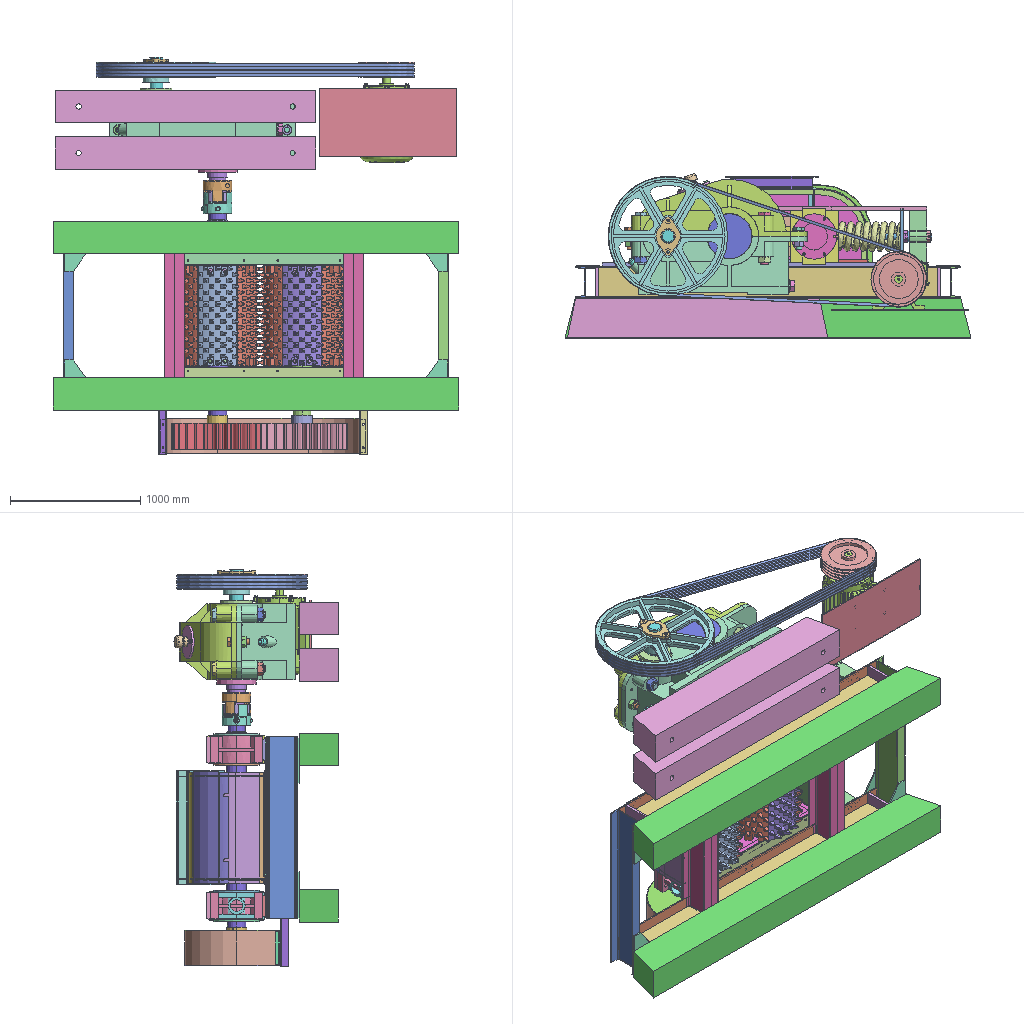Assembly | NX | 107 different items | 209 placed | box 3120 x 1261 x 3058 mm
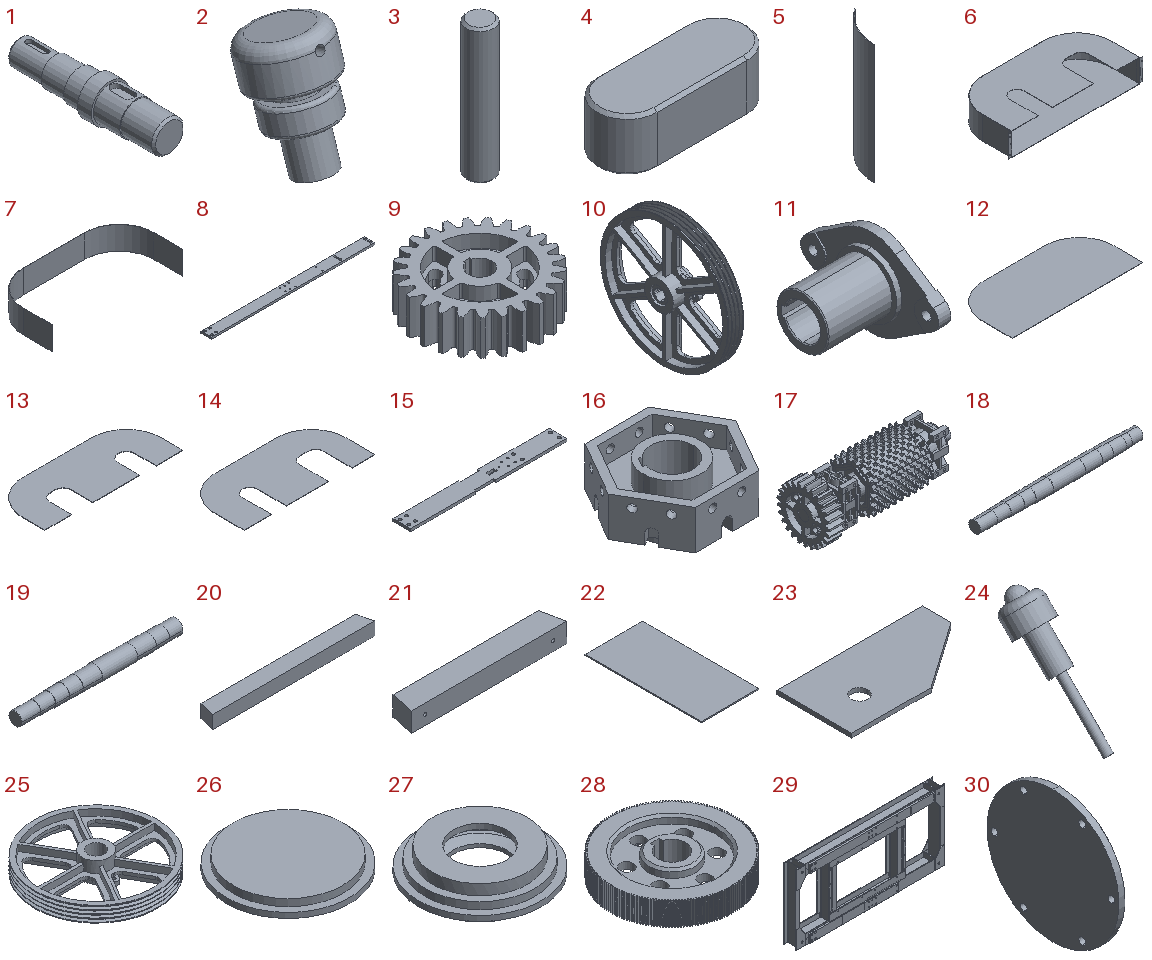Parts list (item | name | quantity | parent item | size | volume | features):
1 | - | x1 | in 84 | 202.5 x 798.75 x 202.5 mm | 16646925 mm3 | features BOSS 5, CHAMFER 2, DATUM_PLANE 2, RECT_SLOT 2, CYLINDER 1, DATUM_CSYS 1, Delete Body 1, LINKED_BODY 1, MOVE_FACE 1, SCALE 1
2 | - | x1 | in 84 | 93.696 x 105.756 x 150.047 mm | 549540 mm3 | features LINKED_BODY 2, DATUM_CSYS 1, Delete Body 1, Resize Face 1
3 | - | x1 | in 84 | 16.875 x 16.875 x 84.375 mm | 18772 mm3 | features LINKED_BODY 2, DATUM_CSYS 1, Delete Body 1
4 | - | x1 | in 84 | 112.5 x 45 x 39.375 mm | 180850 mm3 | features 28.SLDPRT 2, Delete Body 1, LINKED_BODY 1, SCALE 1
5 | - | x2 | in 75 | 160.623 x 300.85 x 860 mm | 907934 mm3 | features BREP 1
6 | - | x1 | - | 1570 x 734 x 271 mm | 7806699 mm3 | features BREP 4, DATUM_CSYS 1, SKETCH 1
7 | - | x1 | in 6 | 1498 x 729 x 265 mm | 2073983 mm3 | features BREP 1
8 | - | x1 | in 29 | 2499 x 158 x 30 mm | 11579104 mm3 | features BREP 1
9 | - | x2 | in 17, 65 | 701.605 x 700.371 x 200 mm | 42253808 mm3 | features BREP 1
10 | - | x1 | - | 178.109 x 915.408 x 915.408 mm | 21519028 mm3 | features BREP 2, SCALE 2, SPLIT BODY 1, UNITE 1
11 | - | x1 | in 10 | 171.496 x 296.82 x 187.986 mm | 1461921 mm3 | features BREP 1, SCALE 1
12 | - | x1 | in 6 | 1492 x 726 x 3 mm | 3047658 mm3 | features BREP 1, DATUM_CSYS 1, SKETCH 1
13 | - | x2 | in 75 | 1420 x 580 x 4 mm | 2620909 mm3 | features BREP 1
14 | - | x1 | in 6 | 1492 x 726 x 3 mm | 2518464 mm3 | features BREP 1
15 | - | x2 | - | 1759 x 200 x 30 mm | 9929100 mm3 | features BREP 1, DATUM_CSYS 1, SKETCH 1
16 | - | x4 | in 17, 65 | 484.974 x 420 x 200 mm | 14525982 mm3 | features BREP 1
17 | - | x1 | - | - | 267145378 mm3 | features BREP 14, MOVE_FACE 4, DATUM_CSYS 3, SKETCH 3
18 | - | x1 | in 17 | 1889 x 162.539 x 165 mm | 34030029 mm3 | features MOVE_FACE 3, BREP 1
19 | - | x1 | in 65 | 1692 x 162.539 x 165 mm | 31180686 mm3 | features BREP 1
20 | - | x2 | - | 3120 x 300 x 250 mm | 228112500 mm3 | features DATUM_CSYS 1, EXTRUDE 1, SKETCH 1
21 | - | x2 | - | 2000 x 300 x 250 mm | 144558518 mm3 | features BREP 1
22 | - | x1 | - | 525 x 1060 x 10 mm | 5565000 mm3 | features MOVE_FACE 3, BREP 1, DATUM_CSYS 1, DELETE FACE 1, SKETCH 1
23 | - | x8 | in 29 | 350 x 180 x 10 mm | 527834 mm3 | features BREP 1, DATUM_CSYS 1, SKETCH 1
24 | - | x1 | in 84 | 57.861 x 160.996 x 160.996 mm | 163265 mm3 | features DATUM_CSYS 2, Delete Body 2, LINKED_BODY 2, BLEND 1, DATUM_PLANE 1, SCALE 1, SKETCH 1, SWP104 1
25 | - | x1 | in 10 | 915.408 x 915.408 x 151.725 mm | 20057107 mm3 | features BREP 1, SCALE 1, SPLIT BODY 1, UNITE 1
26 | - | x1 | in 84 | 393.75 x 393.75 x 39.375 mm | 3155764 mm3 | features CYLINDER 3, DATUM_CSYS 1, Delete Body 1, LINKED_BODY 1, SCALE 1
27 | - | x1 | in 84 | 393.75 x 393.75 x 90 mm | 4276272 mm3 | features SIMPLE HOLE 4, CYLINDER 3, CHAMFER 2, DATUM_CSYS 1, Delete Body 1, LINKED_BODY 1, SCALE 1
28 | - | x1 | in 84 | 784.688 x 784.688 x 146.25 mm | 44829602 mm3 | features BREP 184, META 184, INSTANCE 55, EXTRUDE 6, SKETCH 4, CHAMFER 2, CYLINDER 2, DATUM_CSYS 2, Delete Body 2, EXTRACT_FACE 2, CIRCULAR_ISET 1, FSET 1, Instance Feature 1, LINKED_BODY 1, Mirror Feature 1, REPLACE_FACE 1, Resize Face 1, SCALE 1, SWP104 1, TRANSFORM_ISET 1
29 | - | x1 | - | 2963 x 280 x 1400 mm | 109819651 mm3 | features BREP 14, DATUM_CSYS 3, SKETCH 3, LINKED_FACE 1, REPLACE_FACE 1
30 | - | x1 | in 65 | 45 x 350 x 350 mm | 1642719 mm3 | features BREP 1
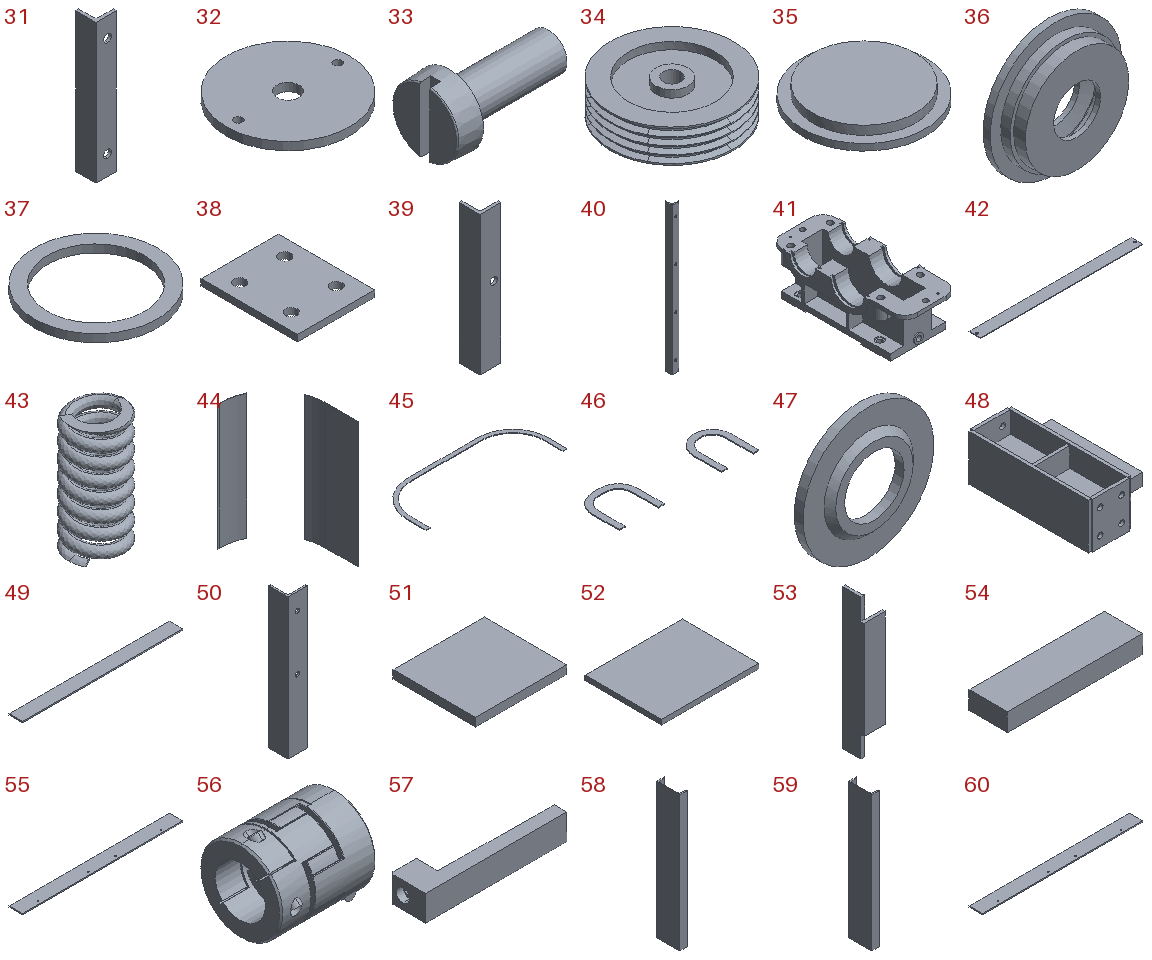31 | - | x2 | in 6 | 36 x 36 x 250 mm | 83297 mm3 | features BREP 1
32 | - | x1 | in 84 | - | 851530 mm3 | features Delete Body 2, LINKED_BODY 2, SIMPLE HOLE 2, SYMBOLIC_THREAD 2, CYLINDER 1, DATUM_CSYS 1, MIRROR_SET 1, SCALE 1, SUBTRACT 1
33 | - | x2 | in 84 | 56.25 x 30.938 x 30.938 mm | 17558 mm3 | features 7.SLDPRT 2, Delete Body 1, LINKED_BODY 1, MOVE_FACE 1, SCALE 1
34 | - | x1 | - | 426.001 x 426 x 114.878 mm | 11128143 mm3 | features DATUM_CSYS 1, LINKED_BODY 1
35 | - | x1 | in 84 | 315 x 315 x 39.375 mm | 2172802 mm3 | features CYLINDER 3, DATUM_CSYS 1, Delete Body 1, LINKED_BODY 1, SCALE 1, UNITE 1
36 | - | x1 | in 84 | 315 x 84.375 x 315 mm | 2887099 mm3 | features SIMPLE HOLE 4, CHAMFER 3, DATUM_CSYS 1, Delete Body 1, LINKED_BODY 1, SCALE 1, SKETCH 1, SWP104 1
37 | - | x2 | in 84 | 264.375 x 264.375 x 16.875 mm | 352256 mm3 | features CYLINDER 2, DATUM_CSYS 1, Delete Body 1, LINKED_BODY 1, SCALE 1
38 | - | x4 | in 48 | 120 x 150 x 10 mm | 169821 mm3 | features BREP 1
39 | - | x2 | in 75 | 40 x 40 x 270 mm | 101929 mm3 | features BREP 1
40 | - | x2 | in 75 | 40 x 40 x 850 mm | 320232 mm3 | features BREP 1
41 | - | x1 | in 84 | 585 x 1429 x 450 mm | 106130816 mm3 | features SKETCH 9, BREP 2, DATUM_PLANE 2, SYMBOLIC_THREAD 2, DATUM_CSYS 1, Delete Body 1, LINKED_BODY 1, REPLACE_FACE 1, UNITE 1
42 | - | x4 | in 29 | 2807 x 200 x 10 mm | 5588867 mm3 | features BREP 1
43 | - | x2 | - | - | 7127986 mm3 | features BREP 1
44 | - | x1 | in 75 | 375 x 583 x 850 mm | 1310584 mm3 | features BREP 2, DATUM_CSYS 1, SKETCH 1
45 | - | x2 | in 75 | 1410 x 540 x 6 mm | 509384 mm3 | features BREP 1
46 | - | x2 | in 75 | 960 x 320 x 6 mm | 357876 mm3 | features BREP 2
47 | - | x2 | in 84 | 247.5 x 28.125 x 247.5 mm | 674318 mm3 | features DATUM_CSYS 1, Delete Body 1, LINKED_BODY 1, SCALE 1, SKETCH 1, SWP104 1
48 | - | x2 | - | 225 x 400 x 150 mm | 3141642 mm3 | features BREP 5
49 | - | x2 | in 29 | 2607 x 220 x 20 mm | 11470800 mm3 | features BREP 1, DATUM_CSYS 1, SKETCH 1
50 | - | x1 | - | 63 x 63 x 460 mm | 280553 mm3 | features BREP 1
51 | - | x4 | in 29 | 220 x 200 x 20 mm | 880000 mm3 | features BREP 1
52 | - | x3 | in 29 | 200 x 158 x 10 mm | 316000 mm3 | features BREP 1
53 | - | x4 | in 75 | 40 x 40 x 265 mm | 84160 mm3 | features BREP 1
54 | - | x2 | in 48 | 300 x 85 x 40 mm | 1020000 mm3 | features BREP 1
55 | - | x1 | in 29 | 1530 x 126 x 10 mm | 1923276 mm3 | features BREP 1
56 | - | x1 | - | 257.704 x 231.242 x 232.662 mm | 6465109 mm3 | features SCALE 4, BREP 3, LINKED_BODY 2, SUBTRACT 2
57 | - | x4 | in 17, 65 | 220 x 55 x 40 mm | 227539 mm3 | features BREP 1
58 | - | x1 | in 29 | 78 x 240 x 1400 mm | 4711916 mm3 | features BREP 1
59 | - | x1 | in 29 | 78 x 240 x 1400 mm | 4711916 mm3 | features BREP 1, LINKED_FACE 1, REPLACE_FACE 1
60 | - | x1 | in 29 | 1530 x 126 x 10 mm | 1923276 mm3 | features BREP 1
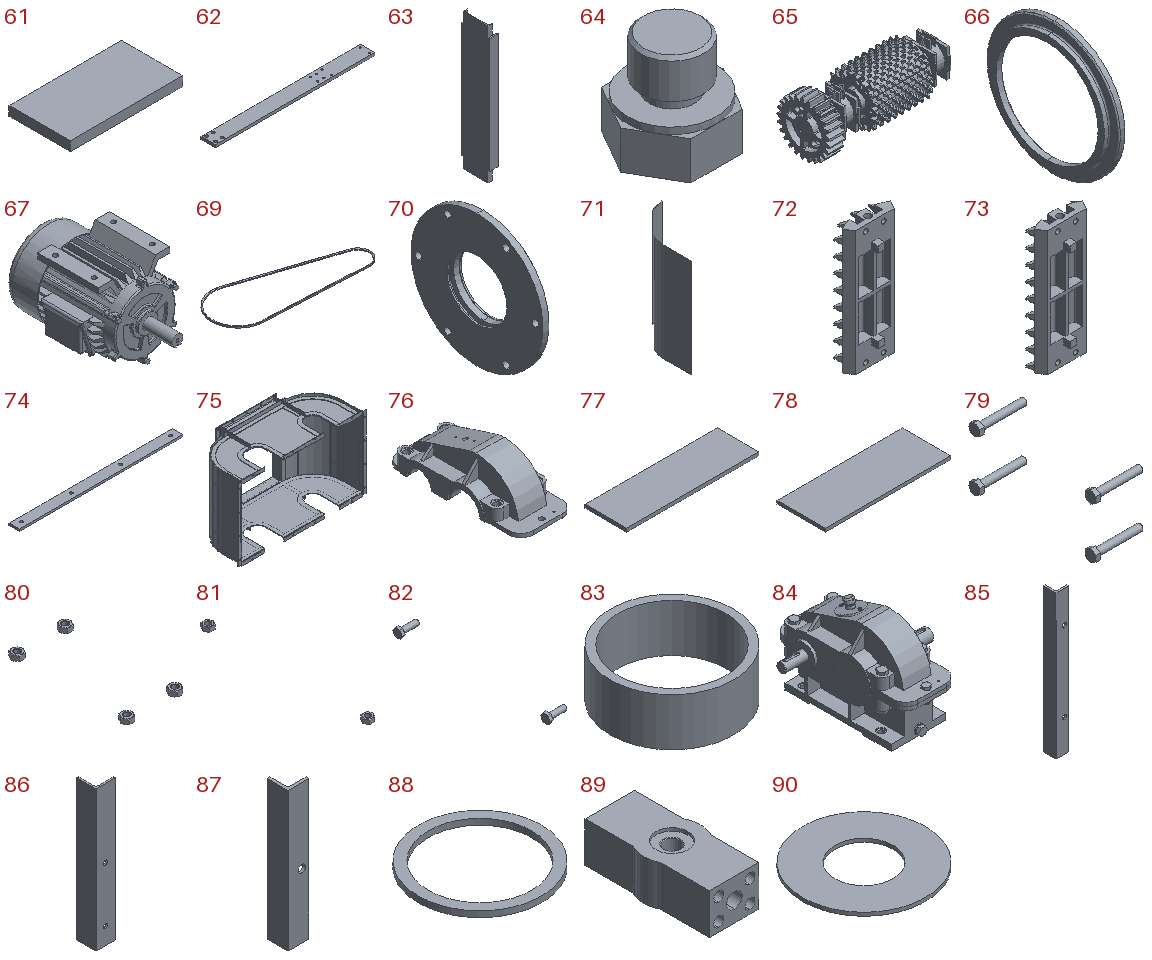61 | - | x4 | in 48 | 120 x 65 x 10 mm | 78000 mm3 | features BREP 1
62 | - | x1 | in 29 | 1764 x 158 x 30 mm | 8203778 mm3 | features BREP 1
63 | - | x4 | in 29 | 78 x 240 x 1180 mm | 3661713 mm3 | features BREP 1, DATUM_CSYS 1, SKETCH 1
64 | - | x1 | in 84 | - | 302869 mm3 | features BOSS 2, CHAMFER 1, CYLINDER 1, DATUM_CSYS 1, Delete Body 1, EXTRUDE 1, LINKED_BODY 1, SCALE 1, SYMBOLIC_THREAD 1
65 | - | x1 | - | - | 260357550 mm3 | features BREP 13, DATUM_CSYS 1, MOVE_FACE 1, SKETCH 1
66 | - | x1 | in 17 | 17 x 195 x 195 mm | 90741 mm3 | features BREP 1
67 | - | x1 | - | 440.662 x 771.03 x 438.512 mm | 51845924 mm3 | features BREP 2, Delete Body 1, EXTRUDE 1, LINKED_FACE 1, REPLACE_FACE 1, SCALE 1, SPLIT BODY 1, UNITE 1
68 | - | x1 | - | - | - | -
69 | - | x4 | - | 2447 x 1004 x 24.054 mm | 1773043 mm3 | features DATUM_CSYS 1, LINKED_BODY 1
70 | - | x4 | in 17, 65 | 45 x 350 x 350 mm | 1918152 mm3 | features BREP 1
71 | - | x1 | in 75 | 325 x 580.972 x 850 mm | 1182499 mm3 | features BREP 2
72 | - | x6 | in 17, 65 | 313.534 x 169.472 x 770 mm | 12152543 mm3 | features BREP 1, DATUM_CSYS 1, SKETCH 1
73 | - | x6 | in 17, 65 | 313.534 x 169.472 x 770 mm | 12115990 mm3 | features BREP 1
74 | - | x2 | in 29 | 790 x 50 x 10 mm | 388842 mm3 | features BREP 1
75 | - | x1 | - | 1506 x 685 x 876 mm | 16741926 mm3 | features BREP 16, DATUM_CSYS 2, SKETCH 2
76 | - | x1 | in 84 | - | 60414139 mm3 | features SKETCH 12, BREP 10, Delete Body 6, MOVE_FACE 5, UNITE 5, BLEND 4, DATUM_CSYS 4, EXTRUDE 4, LINKED_BODY 3, REPLACE_FACE 3, SPLIT BODY 3, SUBTRACT 3, SWP104 3, DATUM_PLANE 2, SYMBOLIC_THREAD 2, ABSOLUTE_DATUM_PLANE 1, Container 1, EXTRACT_BODY 1, Geometry Instance 1, LINE 1
77 | - | x2 | in 48 | 380 x 120 x 10 mm | 456000 mm3 | features BREP 1
78 | - | x4 | in 48 | 390 x 150 x 10 mm | 585000 mm3 | features BREP 1
79 | - | x1 | in 84 | 405.45 x 1039 x 518.419 mm | 4693711 mm3 | features 3.SLDPRT 2, Delete Body 1, LINKED_BODY 1, SCALE 1
80 | - | x1 | in 84 | 520.173 x 1041 x 47.25 mm | 973230 mm3 | features 4.SLDPRT 2, Delete Body 1, LINKED_BODY 1, SCALE 1
81 | - | x1 | in 84 | 84.437 x 1373 x 38.25 mm | 263240 mm3 | features 11.SLDPRT 2, Delete Body 1, LINKED_BODY 1, SCALE 1
82 | - | x1 | in 84 | 170.438 x 1384 x 73.125 mm | 715384 mm3 | features 10.SLDPRT 2, Delete Body 1, LINKED_BODY 1, SCALE 1
83 | - | x3 | in 17, 65 | 160 x 160 x 62 mm | 292168 mm3 | features BREP 1, MOVE_FACE 1
84 | - | x1 | - | - | 277364397 mm3 | features BREP 197, META 184, INSTANCE 70, Delete Body 36, LINKED_BODY 32, SKETCH 29, DATUM_CSYS 23, SCALE 22, CYLINDER 21, CHAMFER 16, BOSS 13, EXTRUDE 12, SIMPLE HOLE 10, UNITE 9, DATUM_PLANE 8, MOVE_FACE 8, SYMBOLIC_THREAD 8, SWP104 7, BLEND 5, REPLACE_FACE 5, SPLIT BODY 5, SUBTRACT 4, RECT_SLOT 3, 10.SLDPRT 2, 11.SLDPRT 2, 25.SLDPRT 2, 28.SLDPRT 2, 29.SLDPRT 2, 3.SLDPRT 2, 4.SLDPRT 2, 7.SLDPRT 2, CIRCULAR_ISET 2, EXTRACT_FACE 2, FSET 2, Resize Face 2, TRANSFORM_ISET 2, ABSOLUTE_DATUM_PLANE 1, Container 1, EXTRACT_BODY 1, Geometry Instance 1, Instance Feature 1, LINE 1, MIRROR 1, MIRROR_SET 1, Mirror Feature 1
85 | - | x2 | in 75 | 40 x 40 x 470 mm | 177232 mm3 | features BREP 1
86 | - | x1 | - | 63 x 63 x 460 mm | 280553 mm3 | features BREP 1
87 | - | x2 | in 75 | 40 x 40 x 270 mm | 101929 mm3 | features BREP 1
88 | - | x1 | in 84 | 348.75 x 348.75 x 16.875 mm | 478061 mm3 | features CYLINDER 2, DATUM_CSYS 1, Delete Body 1, LINKED_BODY 1, SCALE 1
89 | - | x2 | - | 180 x 400 x 130 mm | 6105398 mm3 | features BREP 1
90 | - | x2 | - | 142 x 142 x 4 mm | 49244 mm3 | features BREP 1
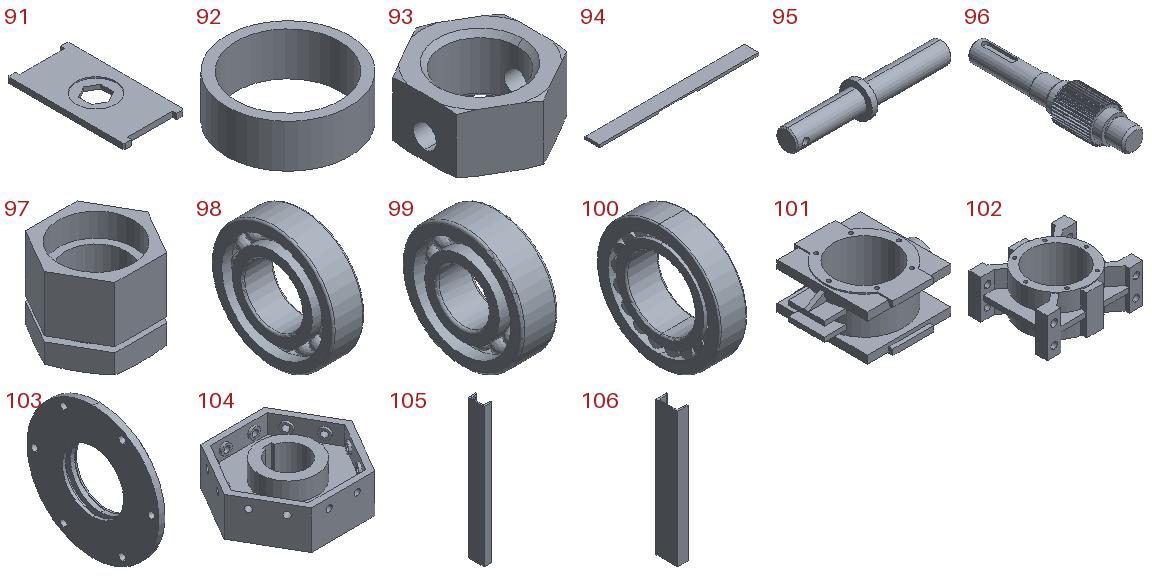91 | - | x2 | - | 220 x 426 x 20 mm | 1605748 mm3 | features BREP 1
92 | - | x1 | in 84 | 208.125 x 208.125 x 73.125 mm | 741414 mm3 | features CYLINDER 2, DATUM_CSYS 1, Delete Body 1, LINKED_BODY 1, SCALE 1
93 | - | x2 | - | 76.6 x 88.249 x 40 mm | 110310 mm3 | features BREP 1
94 | - | x1 | in 29 | 1764 x 158 x 30 mm | 7354110 mm3 | features BREP 1
95 | - | x2 | - | 380 x 80 x 80 mm | 838833 mm3 | features BREP 1
96 | - | x1 | in 84 | - | 9920254 mm3 | features INSTANCE 15, BOSS 6, CHAMFER 6, Delete Body 3, SPLIT BODY 2, UNITE 2, BREP 1, CIRCULAR_ISET 1, CYLINDER 1, DATUM_CSYS 1, DATUM_PLANE 1, EXTRUDE 1, FSET 1, LINKED_BODY 1, MIRROR 1, MOVE_FACE 1, RECT_SLOT 1, SCALE 1, SKETCH 1, SYMBOLIC_THREAD 1, TRANSFORM_ISET 1
97 | - | x2 | - | 88.25 x 76.427 x 70 mm | 175970 mm3 | features BREP 1
98 | - | x2 | in 84 | 90 x 348.75 x 348.75 mm | 4853865 mm3 | features 25.SLDPRT 2, Delete Body 1, LINKED_BODY 1, SCALE 1
99 | - | x2 | in 84 | 78.75 x 264.375 x 264.375 mm | 2601399 mm3 | features 29.SLDPRT 2, Delete Body 1, LINKED_BODY 1, SCALE 1
100 | - | x8 | in 17, 65 | 77 x 270 x 270 mm | 2111667 mm3 | features BREP 1
101 | - | x4 | in 17, 65 | 500 x 436 x 210 mm | 13297149 mm3 | features BREP 1
102 | - | x2 | in 17 | 490 x 400 x 210 mm | 14928889 mm3 | features DATUM_CSYS 2, SKETCH 2, BREP 1
103 | - | x3 | in 17, 65 | 45 x 350 x 350 mm | 1928848 mm3 | features BREP 1
104 | - | x4 | in 17, 65 | 542.709 x 470 x 200 mm | 14287973 mm3 | features BREP 1
105 | - | x2 | in 75 | 48 x 100 x 876 mm | 1087998 mm3 | features BREP 1, DATUM_CSYS 1, SKETCH 1
106 | - | x2 | in 75 | 48 x 100 x 620 mm | 770701 mm3 | features BREP 1
107 | zpt | x1 | - | - | - | -
Mates (type | each side: item.copy, entity, surface, feature):
In the top assembly
Touch | 56.1 face cylinder Body(1) | 1.1 face cylinder Linked Body(15)
Bond | 68.1 component | 22.1 component
Parallel | 22.1 face plane Body(0) | 21.1 face plane Body(1)
Touch | 67.1 face plane Body(0) | 25.1 face plane Body(1)
Fix | 10.1 component
Touch | 67.1 face plane Body(0) | 22.1 face plane Body(0)
In subassembly 10
Touch | 11.1 | 25.1
In subassembly 84
Touch | 99.1 face plane Linked Body(4) | 37.1 face plane Linked Body(5)